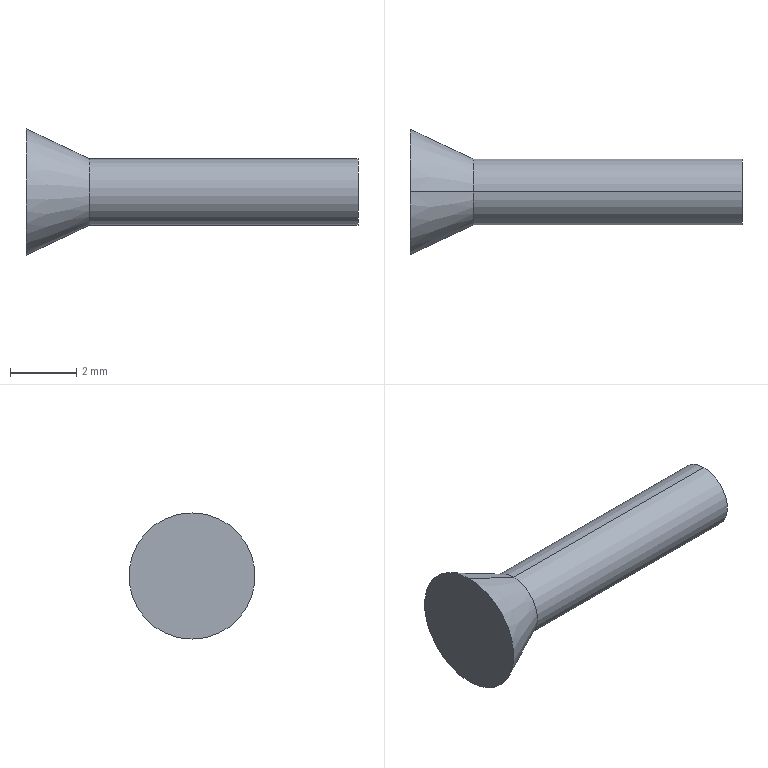Part | SolidWorks | features BaseBody 1 | 1 solid | 6 faces | box 10 x 3.8 x 3.8 mm | volume 38.4 mm3 | cylinder 2 | cone 2 | plane 2 | commonest cylinder face diameters 2 x2
STEP:
#1=CARTESIAN_POINT('',(1.9,0.,-1.));
#2=VERTEX_POINT('',#1);
#3=CARTESIAN_POINT('',(1.9,0.,1.));
#4=VERTEX_POINT('',#3);
#5=CARTESIAN_POINT('',(1.9,0.,0.));
#6=DIRECTION('',(1.,0.,0.));
#7=DIRECTION('',(0.,0.,-1.));
#8=AXIS2_PLACEMENT_3D('',#5,#6,#7);
#9=CIRCLE('',#8,1.);
#10=EDGE_CURVE('',#2,#4,#9,.T.);
#11=ORIENTED_EDGE('',*,*,#10,.T.);
#12=CARTESIAN_POINT('',(10.,0.,1.));
#13=VERTEX_POINT('',#12);
#14=CARTESIAN_POINT('',(10.,0.,1.));
#15=DIRECTION('',(1.,0.,0.));
#16=VECTOR('',#15,1000.);
#17=LINE('',#14,#16);
#18=EDGE_CURVE('',#4,#13,#17,.T.);
#19=ORIENTED_EDGE('',*,*,#18,.T.);
#20=CARTESIAN_POINT('',(10.,0.,-1.));
#21=VERTEX_POINT('',#20);
#22=CARTESIAN_POINT('',(10.,0.,0.));
#23=DIRECTION('',(-1.,0.,0.));
#24=DIRECTION('',(0.,0.,-1.));
#25=AXIS2_PLACEMENT_3D('',#22,#23,#24);
#26=CIRCLE('',#25,1.);
#27=EDGE_CURVE('',#13,#21,#26,.T.);
#28=ORIENTED_EDGE('',*,*,#27,.T.);
#29=CARTESIAN_POINT('',(10.,0.,-1.));
#30=DIRECTION('',(1.,0.,0.));
#31=VECTOR('',#30,1000.);
#32=LINE('',#29,#31);
#33=EDGE_CURVE('',#2,#21,#32,.T.);
#34=ORIENTED_EDGE('',*,*,#33,.F.);
#35=EDGE_LOOP('',(#11,#19,#28,#34));
#36=FACE_OUTER_BOUND('',#35,.T.);
#37=CARTESIAN_POINT('',(10.,0.,0.));
#38=DIRECTION('',(1.,0.,0.));
#39=DIRECTION('',(0.,0.,-1.));
#40=AXIS2_PLACEMENT_3D('',#37,#38,#39);
#41=CYLINDRICAL_SURFACE('',#40,1.);
#42=ADVANCED_FACE('',(#36),#41,.T.);
#43=ORIENTED_EDGE('',*,*,#10,.F.);
#44=CARTESIAN_POINT('',(0.,0.,-1.9));
#45=VERTEX_POINT('',#44);
#46=CARTESIAN_POINT('',(0.,0.,-1.9));
#47=DIRECTION('',(-0.9037,0.,-0.4281));
#48=VECTOR('',#47,1000.);
#49=LINE('',#46,#48);
#50=EDGE_CURVE('',#2,#45,#49,.T.);
#51=ORIENTED_EDGE('',*,*,#50,.T.);
#52=CARTESIAN_POINT('',(0.,0.,1.9));
#53=VERTEX_POINT('',#52);
#54=CARTESIAN_POINT('',(0.,0.,0.));
#55=DIRECTION('',(1.,0.,0.));
#56=DIRECTION('',(0.,0.,1.));
#57=AXIS2_PLACEMENT_3D('',#54,#55,#56);
#58=CIRCLE('',#57,1.9);
#59=EDGE_CURVE('',#45,#53,#58,.T.);
#60=ORIENTED_EDGE('',*,*,#59,.T.);
#61=CARTESIAN_POINT('',(0.,0.,1.9));
#62=DIRECTION('',(-0.9037,0.,0.4281));
#63=VECTOR('',#62,1000.);
#64=LINE('',#61,#63);
#65=EDGE_CURVE('',#4,#53,#64,.T.);
#66=ORIENTED_EDGE('',*,*,#65,.F.);
#67=EDGE_LOOP('',(#43,#51,#60,#66));
#68=FACE_OUTER_BOUND('',#67,.T.);
#69=CARTESIAN_POINT('',(0.,0.,0.));
#70=DIRECTION('',(-1.,0.,0.));
#71=DIRECTION('',(0.,0.,1.));
#72=AXIS2_PLACEMENT_3D('',#69,#70,#71);
#73=CONICAL_SURFACE('',#72,1.9,0.4424);
#74=ADVANCED_FACE('',(#68),#73,.T.);
#75=ORIENTED_EDGE('',*,*,#18,.F.);
#76=CARTESIAN_POINT('',(1.9,0.,0.));
#77=DIRECTION('',(1.,0.,0.));
#78=DIRECTION('',(0.,0.,-1.));
#79=AXIS2_PLACEMENT_3D('',#76,#77,#78);
#80=CIRCLE('',#79,1.);
#81=EDGE_CURVE('',#4,#2,#80,.T.);
#82=ORIENTED_EDGE('',*,*,#81,.T.);
#83=ORIENTED_EDGE('',*,*,#33,.T.);
#84=CARTESIAN_POINT('',(10.,0.,0.));
#85=DIRECTION('',(-1.,0.,0.));
#86=DIRECTION('',(0.,0.,-1.));
#87=AXIS2_PLACEMENT_3D('',#84,#85,#86);
#88=CIRCLE('',#87,1.);
#89=EDGE_CURVE('',#21,#13,#88,.T.);
#90=ORIENTED_EDGE('',*,*,#89,.T.);
#91=EDGE_LOOP('',(#75,#82,#83,#90));
#92=FACE_OUTER_BOUND('',#91,.T.);
#93=CARTESIAN_POINT('',(10.,0.,0.));
#94=DIRECTION('',(1.,0.,0.));
#95=DIRECTION('',(0.,0.,-1.));
#96=AXIS2_PLACEMENT_3D('',#93,#94,#95);
#97=CYLINDRICAL_SURFACE('',#96,1.);
#98=ADVANCED_FACE('',(#92),#97,.T.);
#99=ORIENTED_EDGE('',*,*,#89,.F.);
#100=ORIENTED_EDGE('',*,*,#27,.F.);
#101=EDGE_LOOP('',(#99,#100));
#102=FACE_OUTER_BOUND('',#101,.T.);
#103=CARTESIAN_POINT('',(10.,1.,0.));
#104=DIRECTION('',(-1.,0.,0.));
#105=DIRECTION('',(0.,0.,1.));
#106=AXIS2_PLACEMENT_3D('',#103,#104,#105);
#107=PLANE('',#106);
#108=ADVANCED_FACE('',(#102),#107,.F.);
#109=ORIENTED_EDGE('',*,*,#50,.F.);
#110=ORIENTED_EDGE('',*,*,#81,.F.);
#111=ORIENTED_EDGE('',*,*,#65,.T.);
#112=CARTESIAN_POINT('',(0.,0.,0.));
#113=DIRECTION('',(1.,0.,0.));
#114=DIRECTION('',(0.,0.,1.));
#115=AXIS2_PLACEMENT_3D('',#112,#113,#114);
#116=CIRCLE('',#115,1.9);
#117=EDGE_CURVE('',#53,#45,#116,.T.);
#118=ORIENTED_EDGE('',*,*,#117,.T.);
#119=EDGE_LOOP('',(#109,#110,#111,#118));
#120=FACE_OUTER_BOUND('',#119,.T.);
#121=CARTESIAN_POINT('',(0.,0.,0.));
#122=DIRECTION('',(-1.,0.,0.));
#123=DIRECTION('',(0.,0.,1.));
#124=AXIS2_PLACEMENT_3D('',#121,#122,#123);
#125=CONICAL_SURFACE('',#124,1.9,0.4424);
#126=ADVANCED_FACE('',(#120),#125,.T.);
#127=ORIENTED_EDGE('',*,*,#117,.F.);
#128=ORIENTED_EDGE('',*,*,#59,.F.);
#129=EDGE_LOOP('',(#127,#128));
#130=FACE_OUTER_BOUND('',#129,.T.);
#131=CARTESIAN_POINT('',(0.,0.,0.));
#132=DIRECTION('',(1.,0.,0.));
#133=DIRECTION('',(0.,0.,-1.));
#134=AXIS2_PLACEMENT_3D('',#131,#132,#133);
#135=PLANE('',#134);
#136=ADVANCED_FACE('',(#130),#135,.F.);
#137=CLOSED_SHELL('',(#42,#74,#98,#108,#126,#136));
#138=MANIFOLD_SOLID_BREP('',#137);
#139=CARTESIAN_POINT('',(0.,0.,0.));
#140=DIRECTION('',(0.,0.,1.));
#141=DIRECTION('',(1.,0.,0.));
#142=AXIS2_PLACEMENT_3D('',#139,#140,#141);
#143=(LENGTH_UNIT()NAMED_UNIT(*)SI_UNIT(.MILLI.,.METRE.));
#144=UNCERTAINTY_MEASURE_WITH_UNIT(LENGTH_MEASURE(0.00001),#143,'','');
#145=(NAMED_UNIT(*)PLANE_ANGLE_UNIT()SI_UNIT($,.RADIAN.));
#146=(NAMED_UNIT(*)SI_UNIT($,.STERADIAN.)SOLID_ANGLE_UNIT());
#147=(GEOMETRIC_REPRESENTATION_CONTEXT(3)GLOBAL_UNCERTAINTY_ASSIGNED_CONTEXT((#144))GLOBAL_UNIT_ASSIGNED_CONTEXT((#143,#145,#146))REPRESENTATION_CONTEXT('',''));
#148=ADVANCED_BREP_SHAPE_REPRESENTATION('',(#138,#142),#147);